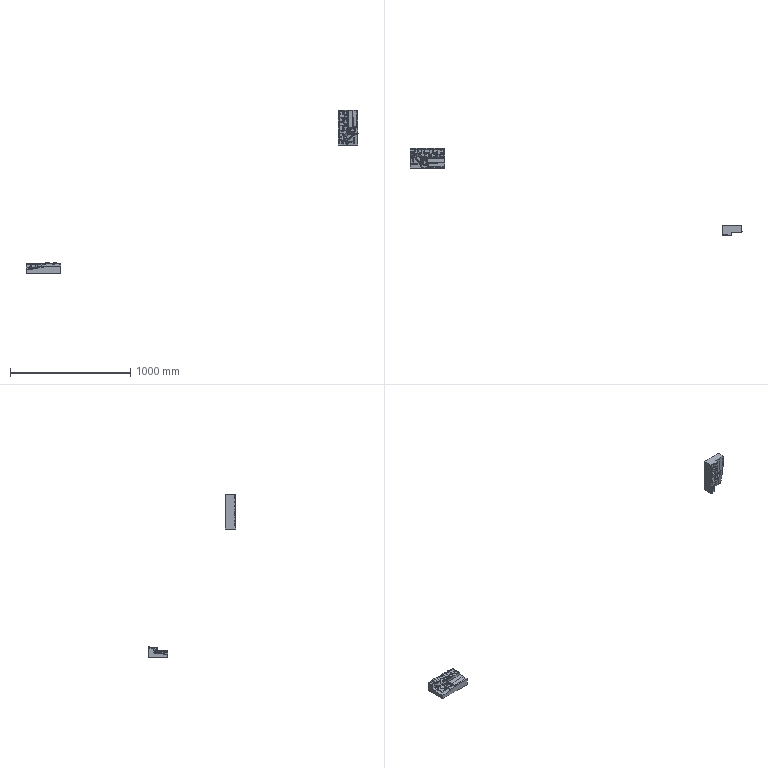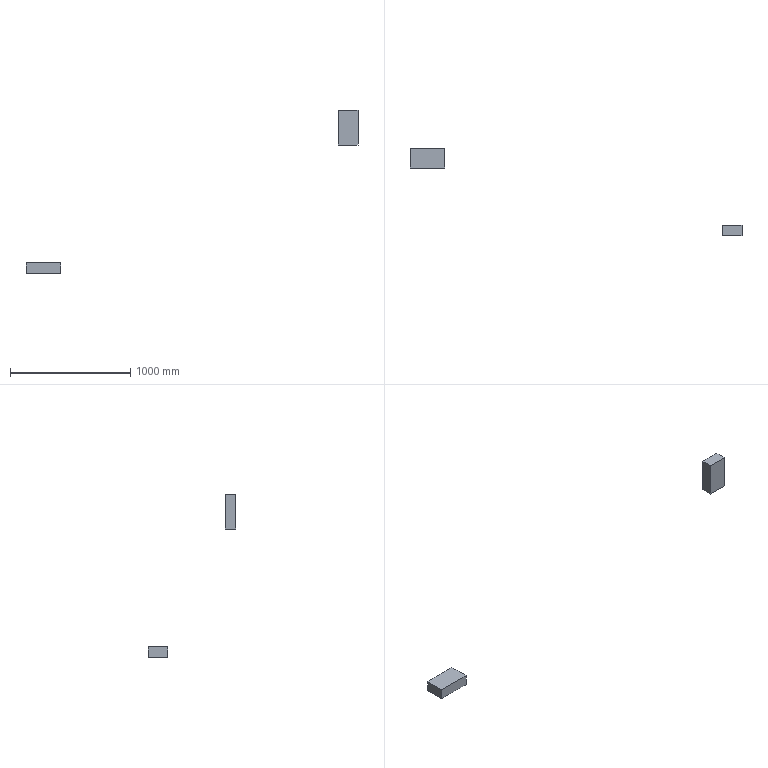CAM job | NX | 3+2 milling | part box 2756 x 729.572 x 1353 mm | stock box 2756 x 729.822 x 1353 mm
Tools:
number,name,description,diameter,corner_radius,flute_length,length,flutes
0,D30R5,Milling Tool-5 Parameters,30.0,5.0,50.0,75.0,2
0,D12,Milling Tool-5 Parameters,12.0,0.0,50.0,75.0,2
0,B10,Milling Tool-Ball Mill,10.0,5.0,50.0,75.0,2
0,B6,Milling Tool-Ball Mill,6.0,3.0,50.0,75.0,2
0,B4,Milling Tool-Ball Mill,4.0,2.0,50.0,75.0,2
0,D6R3,Milling Tool-5 Parameters,6.0,3.0,50.0,75.0,2
Operations:
program,operation,operation_type,tool,method,geometry_group,spindle_rpm,surface_speed,feed_per_tooth,feed_cut,feed_plunge,cut_length_mm,path_length_mm,cut_time_min,machine_time_min
PROGRAM,CAVITY_MILL,CavityMilling,D30R5,METHOD,WORKPIECE,3000.0,282.0,0.4167,2500.0,100.0,173460.176,175912.989,69.384,69.629
PROGRAM,CAVITY_MILL_COPY,CavityMilling,D12,METHOD,WORKPIECE,3000.0,282.0,0.4167,2500.0,100.0,21999.941,38331.204,8.8,10.433
PROGRAM,ZLEVEL_PROFILE,ZLevelMilling,D12,METHOD,WORKPIECE,3000.0,282.0,0.4167,2500.0,100.0,68167.024,73452.962,27.267,27.795
PROGRAM,CONTOUR_AREA,SurfaceContour,B10,METHOD,WORKPIECE,3000.0,282.0,0.4167,2500.0,100.0,18065.321,18083.321,7.226,7.228
PROGRAM,STREAMLINE,SurfaceContour,B6,METHOD,MCS_MILL,3000.0,282.0,0.4167,2500.0,100.0,7372.462,7396.462,2.949,2.951
PROGRAM,CONTOUR_AREA_1,SurfaceContour,B10,METHOD,WORKPIECE,3000.0,282.0,0.4167,2500.0,100.0,91994.493,92020.493,36.798,36.8
PROGRAM,CONTOUR_AREA_2,SurfaceContour,B4,METHOD,WORKPIECE,3000.0,282.0,0.4167,2500.0,100.0,12303.951,12332.751,4.922,4.925
PROGRAM,ZLEVEL_PROFILE_1,ZLevelMilling,B10,METHOD,WORKPIECE,3000.0,282.0,0.4167,2500.0,100.0,60336.106,64530.869,24.134,24.554
PROGRAM,CONTOUR_AREA_4,SurfaceContour,B10,METHOD,WORKPIECE,3000.0,282.0,0.4167,2500.0,100.0,130596.176,130672.176,52.239,52.246
PROGRAM,CONTOUR_AREA_2_COPY,SurfaceContour,B4,METHOD,WORKPIECE,3000.0,282.0,0.4167,2500.0,100.0,7461.561,7513.561,2.985,2.99
LXB,CAVITY_MILL_1,CavityMilling,D30R5,METHOD,W2,3000.0,282.0,0.4167,2500.0,100.0,380983.427,389647.477,152.393,153.26
LXB,CAVITY_MILL_1_COPY,CavityMilling,D12,METHOD,W2,3000.0,282.0,0.4167,2500.0,100.0,21947.841,37528.313,8.779,10.337
LXB,ZLEVEL_PROFILE_2,ZLevelMilling,D12,METHOD,W2,3000.0,282.0,0.4167,2500.0,100.0,342279.286,345716.187,136.912,137.255
LXB,CAVITY_MILL_1_COPY_COPY,CavityMilling,D6R3,METHOD,W2,3000.0,282.0,0.4167,2500.0,100.0,4276.612,7021.839,1.711,1.985
LXB,ZLEVEL_PROFILE_3,ZLevelMilling,D12,METHOD,W2,3000.0,282.0,0.4167,2500.0,100.0,44900.705,47363.78,17.96,18.207
LXB,FIXED_CONTOUR,SurfaceContour,B6,METHOD,W2,3000.0,282.0,0.4167,2500.0,100.0,3564.773,3585.173,1.426,1.428